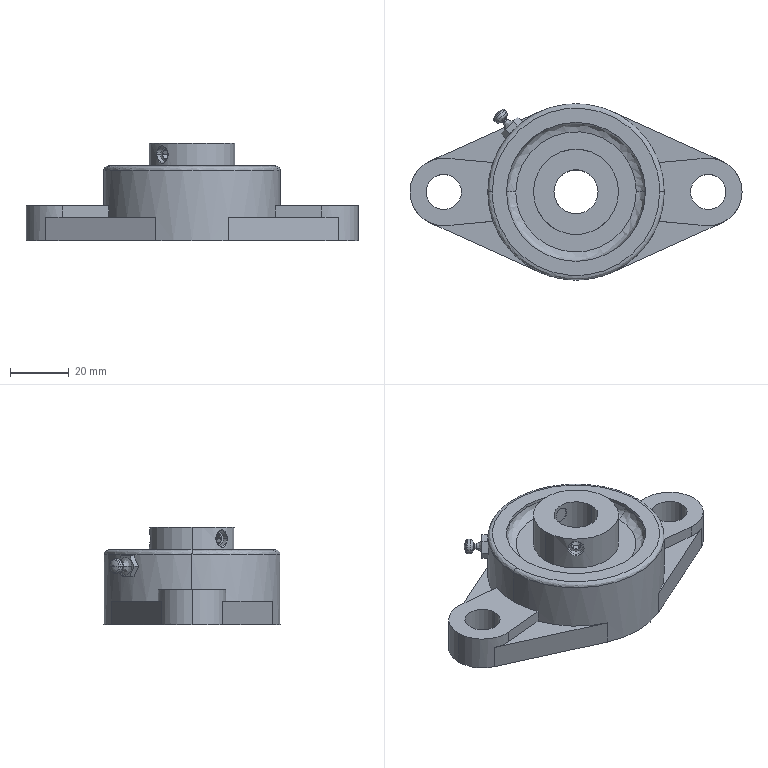Part | SolidWorks | features Simplified 1 | 3 solids | 139 faces | box 113 x 60 x 33.3 mm | volume 71709 mm3 | plane 58 | cone 32 | cylinder 31 | spline 18 | commonest cylinder face diameters 5.188 x4 6 x4 12 x4 47.3 x4 23 x3 2 x2